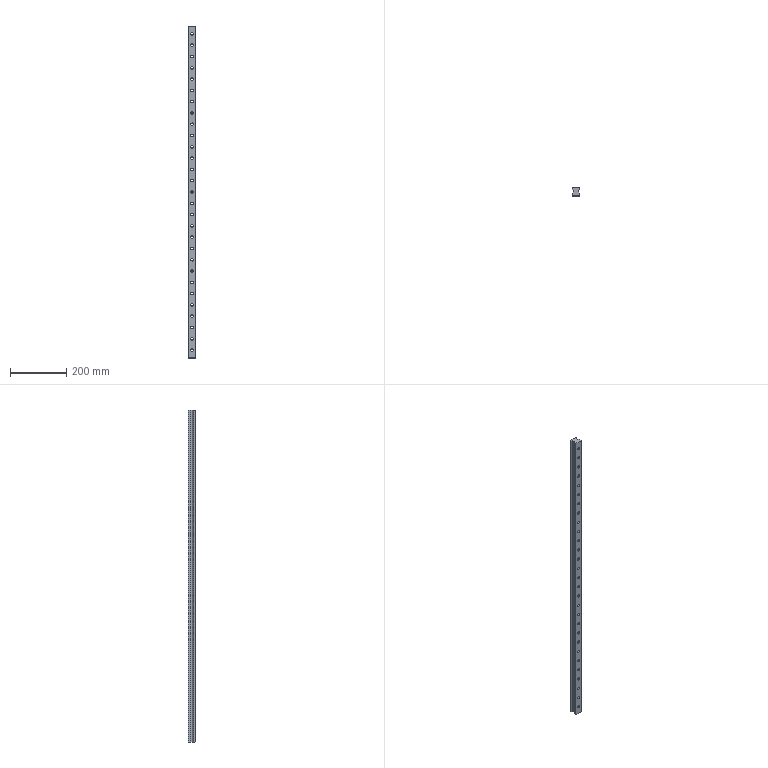Part | SolidWorks | features BaseBody 1 | 1 solid | 161 faces | box 28 x 28 x 1176 mm | volume 695129 mm3 | cylinder 116 | plane 45 | commonest cylinder face diameters 9 x58 14 x58